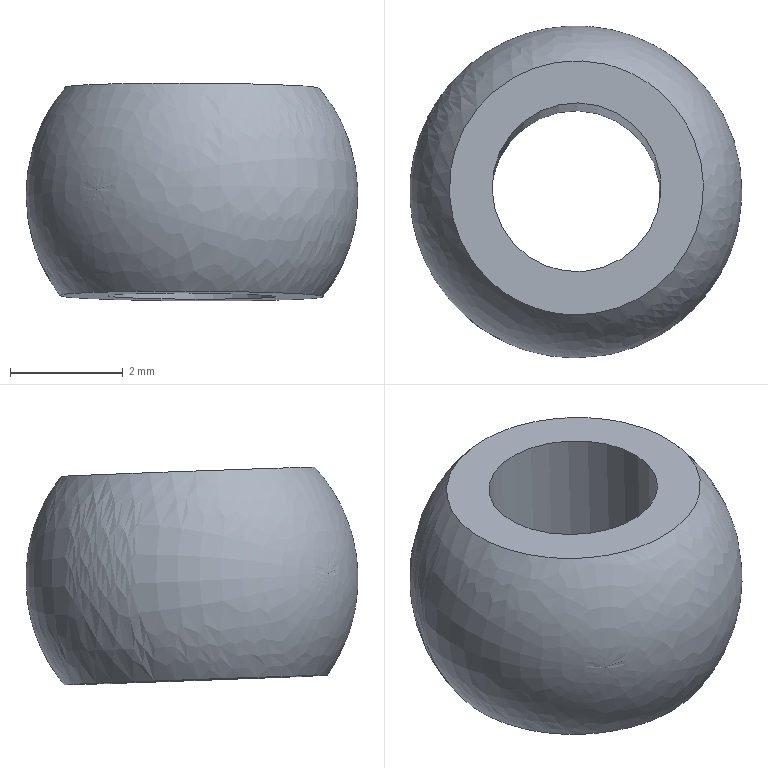Part | STEP file | Wytnij-wyci_gni_cie1_2 | 1 solid | 4 faces | volume 61.693 mm3 | plane 2 | spline 1 | cylinder 1 | commonest cylinder face diameters 3 x1